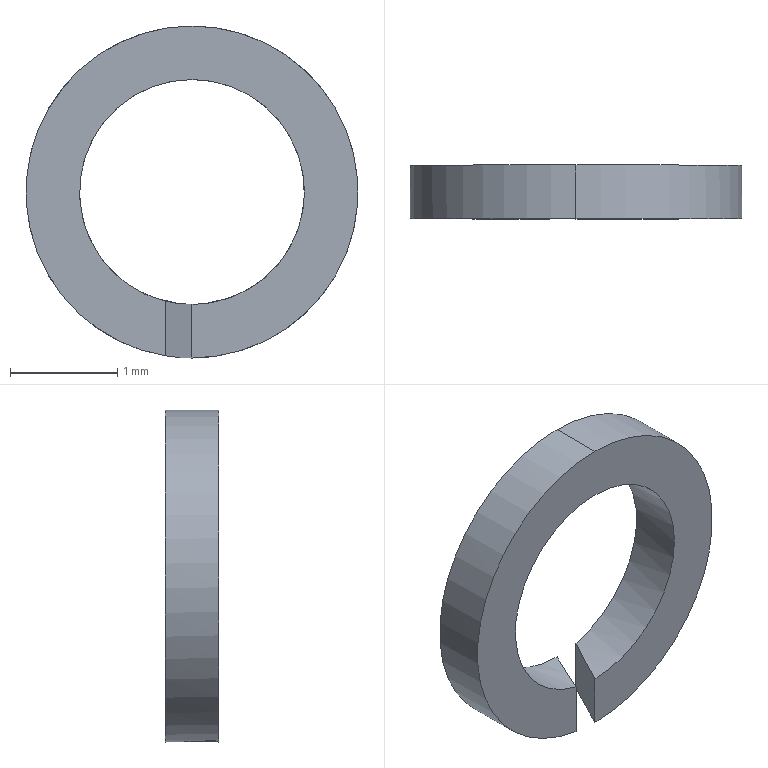Part | STEP file | _1-SO-80980001_1_1_1 | 1 solid | 8 faces | box 3.1 x 0.5 x 3.1 mm | volume 1.979 mm3 | cylinder 4 | plane 4 | commonest cylinder face diameters 2.1 x2 3.1 x2
STEP:
#1=CARTESIAN_POINT('',(0.,0.,0.));
#2=DIRECTION('',(0.,0.,1.));
#3=DIRECTION('',(1.,0.,0.));
#4=AXIS2_PLACEMENT_3D('',#1,#2,#3);
#5=CARTESIAN_POINT('',(-1.75,40.9,-83.78));
#6=VERTEX_POINT('',#5);
#7=CARTESIAN_POINT('',(-1.5,40.9,-80.7));
#8=VERTEX_POINT('',#7);
#9=CARTESIAN_POINT('',(-1.5,40.9,-82.25));
#10=DIRECTION('',(0.,1.,0.));
#11=DIRECTION('',(0.,0.,1.));
#12=AXIS2_PLACEMENT_3D('',#9,#10,#11);
#13=CIRCLE('',#12,1.55);
#14=CARTESIAN_POINT('',(-1.5,40.9,-82.25));
#15=DIRECTION('',(0.,1.,0.));
#16=DIRECTION('',(0.,0.,1.));
#17=AXIS2_PLACEMENT_3D('',#14,#15,#16);
#18=CYLINDRICAL_SURFACE('',#17,1.55);
#19=CARTESIAN_POINT('',(0.,0.));
#20=DIRECTION('',(1.,0.));
#21=VECTOR('',#20,1.);
#22=LINE('',#19,#21);
#23=(GEOMETRIC_REPRESENTATION_CONTEXT(2)PARAMETRIC_REPRESENTATION_CONTEXT()REPRESENTATION_CONTEXT('',''));
#24=DEFINITIONAL_REPRESENTATION('',(#22),#23);
#25=PCURVE('',#18,#24);
#26=CARTESIAN_POINT('',(-1.5,40.9,-82.25));
#27=DIRECTION('',(0.,1.,0.));
#28=DIRECTION('',(0.,0.,1.));
#29=AXIS2_PLACEMENT_3D('',#26,#27,#28);
#30=PLANE('',#29);
#31=CARTESIAN_POINT('',(0.,0.));
#32=DIRECTION('',(1.,0.));
#33=AXIS2_PLACEMENT_2D('',#31,#32);
#34=CIRCLE('',#33,1.55);
#35=(GEOMETRIC_REPRESENTATION_CONTEXT(2)PARAMETRIC_REPRESENTATION_CONTEXT()REPRESENTATION_CONTEXT('',''));
#36=DEFINITIONAL_REPRESENTATION('',(#34),#35);
#37=PCURVE('',#30,#36);
#38=SURFACE_CURVE('',#13,(#25,#37),.PCURVE_S1.);
#39=EDGE_CURVE('',#6,#8,#38,.T.);
#40=ORIENTED_EDGE('',*,*,#39,.T.);
#41=CARTESIAN_POINT('',(-1.5,41.4,-80.7));
#42=VERTEX_POINT('',#41);
#43=CARTESIAN_POINT('',(-1.5,40.9,-80.7));
#44=DIRECTION('',(0.,1.,0.));
#45=VECTOR('',#44,1.);
#46=LINE('',#43,#45);
#47=CARTESIAN_POINT('',(6.283,0.));
#48=DIRECTION('',(0.,1.));
#49=VECTOR('',#48,1.);
#50=LINE('',#47,#49);
#51=(GEOMETRIC_REPRESENTATION_CONTEXT(2)PARAMETRIC_REPRESENTATION_CONTEXT()REPRESENTATION_CONTEXT('',''));
#52=DEFINITIONAL_REPRESENTATION('',(#50),#51);
#53=PCURVE('',#18,#52);
#54=CARTESIAN_POINT('',(-1.5,40.9,-82.25));
#55=DIRECTION('',(0.,1.,0.));
#56=DIRECTION('',(0.,0.,1.));
#57=AXIS2_PLACEMENT_3D('',#54,#55,#56);
#58=CYLINDRICAL_SURFACE('',#57,1.55);
#59=CARTESIAN_POINT('',(0.,0.));
#60=DIRECTION('',(0.,1.));
#61=VECTOR('',#60,1.);
#62=LINE('',#59,#61);
#63=(GEOMETRIC_REPRESENTATION_CONTEXT(2)PARAMETRIC_REPRESENTATION_CONTEXT()REPRESENTATION_CONTEXT('',''));
#64=DEFINITIONAL_REPRESENTATION('',(#62),#63);
#65=PCURVE('',#58,#64);
#66=SURFACE_CURVE('',#46,(#53,#65),.PCURVE_S1.);
#67=EDGE_CURVE('',#8,#42,#66,.T.);
#68=ORIENTED_EDGE('',*,*,#67,.T.);
#69=CARTESIAN_POINT('',(-1.5,41.4,-83.8));
#70=VERTEX_POINT('',#69);
#71=CARTESIAN_POINT('',(-1.5,41.4,-82.25));
#72=DIRECTION('',(0.,1.,0.));
#73=DIRECTION('',(0.,0.,1.));
#74=AXIS2_PLACEMENT_3D('',#71,#72,#73);
#75=CIRCLE('',#74,1.55);
#76=CARTESIAN_POINT('',(0.,0.5));
#77=DIRECTION('',(1.,0.));
#78=VECTOR('',#77,1.);
#79=LINE('',#76,#78);
#80=(GEOMETRIC_REPRESENTATION_CONTEXT(2)PARAMETRIC_REPRESENTATION_CONTEXT()REPRESENTATION_CONTEXT('',''));
#81=DEFINITIONAL_REPRESENTATION('',(#79),#80);
#82=PCURVE('',#18,#81);
#83=CARTESIAN_POINT('',(-1.5,41.4,-82.25));
#84=DIRECTION('',(0.,1.,0.));
#85=DIRECTION('',(0.,0.,1.));
#86=AXIS2_PLACEMENT_3D('',#83,#84,#85);
#87=PLANE('',#86);
#88=CARTESIAN_POINT('',(0.,0.));
#89=DIRECTION('',(1.,0.));
#90=AXIS2_PLACEMENT_2D('',#88,#89);
#91=CIRCLE('',#90,1.55);
#92=(GEOMETRIC_REPRESENTATION_CONTEXT(2)PARAMETRIC_REPRESENTATION_CONTEXT()REPRESENTATION_CONTEXT('',''));
#93=DEFINITIONAL_REPRESENTATION('',(#91),#92);
#94=PCURVE('',#87,#93);
#95=SURFACE_CURVE('',#75,(#82,#94),.PCURVE_S1.);
#96=EDGE_CURVE('',#70,#42,#95,.T.);
#97=ORIENTED_EDGE('',*,*,#96,.F.);
#98=CARTESIAN_POINT('',(-1.5,41.4,-83.8));
#99=CARTESIAN_POINT('',(-1.584,41.232,-83.8));
#100=CARTESIAN_POINT('',(-1.667,41.065,-83.793));
#101=CARTESIAN_POINT('',(-1.75,40.9,-83.78));
#102=(BOUNDED_CURVE()B_SPLINE_CURVE(3,(#98,#99,#100,#101),.UNSPECIFIED.,.F.,.F.)B_SPLINE_CURVE_WITH_KNOTS((4,4),(1.571,1.733),.PIECEWISE_BEZIER_KNOTS.)CURVE()GEOMETRIC_REPRESENTATION_ITEM()RATIONAL_B_SPLINE_CURVE((1.,0.9978,0.9978,1.))REPRESENTATION_ITEM(''));
#103=CARTESIAN_POINT('',(3.142,0.5));
#104=CARTESIAN_POINT('',(3.144,0.4924));
#105=CARTESIAN_POINT('',(3.149,0.4772));
#106=CARTESIAN_POINT('',(3.156,0.4544));
#107=CARTESIAN_POINT('',(3.164,0.4316));
#108=CARTESIAN_POINT('',(3.171,0.4088));
#109=CARTESIAN_POINT('',(3.178,0.3859));
#110=CARTESIAN_POINT('',(3.186,0.3631));
#111=CARTESIAN_POINT('',(3.193,0.3403));
#112=CARTESIAN_POINT('',(3.2,0.3175));
#113=CARTESIAN_POINT('',(3.208,0.2947));
#114=CARTESIAN_POINT('',(3.215,0.2719));
#115=CARTESIAN_POINT('',(3.223,0.2492));
#116=CARTESIAN_POINT('',(3.23,0.2264));
#117=CARTESIAN_POINT('',(3.237,0.2037));
#118=CARTESIAN_POINT('',(3.245,0.181));
#119=CARTESIAN_POINT('',(3.252,0.1582));
#120=CARTESIAN_POINT('',(3.259,0.1356));
#121=CARTESIAN_POINT('',(3.267,0.1129));
#122=CARTESIAN_POINT('',(3.274,0.09026));
#123=CARTESIAN_POINT('',(3.282,0.06765));
#124=CARTESIAN_POINT('',(3.289,0.04507));
#125=CARTESIAN_POINT('',(3.296,0.02251));
#126=CARTESIAN_POINT('',(3.301,0.007501));
#127=CARTESIAN_POINT('',(3.304,0.));
#128=B_SPLINE_CURVE_WITH_KNOTS('',3,(#103,#104,#105,#106,#107,#108,#109,#110,#111,#112,#113,#114,#115,#116,#117,#118,#119,#120,#121,#122,#123,#124,#125,#126,#127),.UNSPECIFIED.,.F.,.F.,(4,1,1,1,1,1,1,1,1,1,1,1,1,1,1,1,1,1,1,1,1,1,4),(1.571,1.578,1.586,1.593,1.6,1.608,1.615,1.622,1.63,1.637,1.644,1.652,1.659,1.667,1.674,1.681,1.689,1.696,1.703,1.711,1.718,1.725,1.733),.QUASI_UNIFORM_KNOTS.);
#129=(GEOMETRIC_REPRESENTATION_CONTEXT(2)PARAMETRIC_REPRESENTATION_CONTEXT()REPRESENTATION_CONTEXT('',''));
#130=DEFINITIONAL_REPRESENTATION('',(#128),#129);
#131=PCURVE('',#18,#130);
#132=CARTESIAN_POINT('',(-1.75,40.9,-82.25));
#133=DIRECTION('',(-0.8944,0.4472,0.));
#134=DIRECTION('',(-0.4472,-0.8944,0.));
#135=AXIS2_PLACEMENT_3D('',#132,#133,#134);
#136=PLANE('',#135);
#137=CARTESIAN_POINT('',(-0.559,-1.55));
#138=CARTESIAN_POINT('',(-0.3717,-1.55));
#139=CARTESIAN_POINT('',(-0.1849,-1.543));
#140=CARTESIAN_POINT('',(0.,-1.53));
#141=(BOUNDED_CURVE()B_SPLINE_CURVE(3,(#137,#138,#139,#140),.UNSPECIFIED.,.F.,.F.)B_SPLINE_CURVE_WITH_KNOTS((4,4),(1.571,1.733),.PIECEWISE_BEZIER_KNOTS.)CURVE()GEOMETRIC_REPRESENTATION_ITEM()RATIONAL_B_SPLINE_CURVE((1.,0.9978,0.9978,1.))REPRESENTATION_ITEM(''));
#142=(GEOMETRIC_REPRESENTATION_CONTEXT(2)PARAMETRIC_REPRESENTATION_CONTEXT()REPRESENTATION_CONTEXT('',''));
#143=DEFINITIONAL_REPRESENTATION('',(#141),#142);
#144=PCURVE('',#136,#143);
#145=SURFACE_CURVE('',#102,(#131,#144),.PCURVE_S1.);
#146=EDGE_CURVE('',#70,#6,#145,.T.);
#147=ORIENTED_EDGE('',*,*,#146,.T.);
#148=EDGE_LOOP('',(#40,#68,#97,#147));
#149=FACE_BOUND('',#148,.T.);
#150=ADVANCED_FACE('',(#149),#18,.T.);
#151=CARTESIAN_POINT('',(-1.5,40.9,-83.3));
#152=VERTEX_POINT('',#151);
#153=CARTESIAN_POINT('',(-1.25,41.4,-83.27));
#154=VERTEX_POINT('',#153);
#155=CARTESIAN_POINT('',(-1.5,40.9,-83.3));
#156=CARTESIAN_POINT('',(-1.416,41.069,-83.3));
#157=CARTESIAN_POINT('',(-1.332,41.236,-83.29));
#158=CARTESIAN_POINT('',(-1.25,41.4,-83.27));
#159=(BOUNDED_CURVE()B_SPLINE_CURVE(3,(#155,#156,#157,#158),.UNSPECIFIED.,.F.,.F.)B_SPLINE_CURVE_WITH_KNOTS((4,4),(4.712,4.953),.PIECEWISE_BEZIER_KNOTS.)CURVE()GEOMETRIC_REPRESENTATION_ITEM()RATIONAL_B_SPLINE_CURVE((1.,0.9952,0.9952,1.))REPRESENTATION_ITEM(''));
#160=CARTESIAN_POINT('',(-1.5,40.9,-82.25));
#161=DIRECTION('',(0.,1.,0.));
#162=DIRECTION('',(0.,0.,1.));
#163=AXIS2_PLACEMENT_3D('',#160,#161,#162);
#164=CYLINDRICAL_SURFACE('',#163,1.05);
#165=CARTESIAN_POINT('',(3.142,0.));
#166=CARTESIAN_POINT('',(3.138,0.007631));
#167=CARTESIAN_POINT('',(3.131,0.0229));
#168=CARTESIAN_POINT('',(3.12,0.04581));
#169=CARTESIAN_POINT('',(3.109,0.06873));
#170=CARTESIAN_POINT('',(3.098,0.09165));
#171=CARTESIAN_POINT('',(3.087,0.1146));
#172=CARTESIAN_POINT('',(3.076,0.1375));
#173=CARTESIAN_POINT('',(3.065,0.1604));
#174=CARTESIAN_POINT('',(3.054,0.1833));
#175=CARTESIAN_POINT('',(3.043,0.2061));
#176=CARTESIAN_POINT('',(3.032,0.229));
#177=CARTESIAN_POINT('',(3.021,0.2518));
#178=CARTESIAN_POINT('',(3.01,0.2746));
#179=CARTESIAN_POINT('',(3.,0.2974));
#180=CARTESIAN_POINT('',(2.989,0.3201));
#181=CARTESIAN_POINT('',(2.978,0.3428));
#182=CARTESIAN_POINT('',(2.967,0.3654));
#183=CARTESIAN_POINT('',(2.956,0.388));
#184=CARTESIAN_POINT('',(2.945,0.4105));
#185=CARTESIAN_POINT('',(2.934,0.433));
#186=CARTESIAN_POINT('',(2.923,0.4554));
#187=CARTESIAN_POINT('',(2.912,0.4777));
#188=CARTESIAN_POINT('',(2.905,0.4926));
#189=CARTESIAN_POINT('',(2.901,0.5));
#190=B_SPLINE_CURVE_WITH_KNOTS('',3,(#165,#166,#167,#168,#169,#170,#171,#172,#173,#174,#175,#176,#177,#178,#179,#180,#181,#182,#183,#184,#185,#186,#187,#188,#189),.UNSPECIFIED.,.F.,.F.,(4,1,1,1,1,1,1,1,1,1,1,1,1,1,1,1,1,1,1,1,1,1,4),(4.712,4.723,4.734,4.745,4.756,4.767,4.778,4.789,4.8,4.811,4.822,4.833,4.844,4.854,4.865,4.876,4.887,4.898,4.909,4.92,4.931,4.942,4.953),.QUASI_UNIFORM_KNOTS.);
#191=(GEOMETRIC_REPRESENTATION_CONTEXT(2)PARAMETRIC_REPRESENTATION_CONTEXT()REPRESENTATION_CONTEXT('',''));
#192=DEFINITIONAL_REPRESENTATION('',(#190),#191);
#193=PCURVE('',#164,#192);
#194=CARTESIAN_POINT('',(-1.25,41.4,-82.25));
#195=DIRECTION('',(0.8944,-0.4472,0.));
#196=DIRECTION('',(0.4472,0.8944,0.));
#197=AXIS2_PLACEMENT_3D('',#194,#195,#196);
#198=PLANE('',#197);
#199=CARTESIAN_POINT('',(-0.559,-1.05));
#200=CARTESIAN_POINT('',(-0.3704,-1.05));
#201=CARTESIAN_POINT('',(-0.1832,-1.04));
#202=CARTESIAN_POINT('',(0.,-1.02));
#203=(BOUNDED_CURVE()B_SPLINE_CURVE(3,(#199,#200,#201,#202),.UNSPECIFIED.,.F.,.F.)B_SPLINE_CURVE_WITH_KNOTS((4,4),(4.712,4.953),.PIECEWISE_BEZIER_KNOTS.)CURVE()GEOMETRIC_REPRESENTATION_ITEM()RATIONAL_B_SPLINE_CURVE((1.,0.9952,0.9952,1.))REPRESENTATION_ITEM(''));
#204=(GEOMETRIC_REPRESENTATION_CONTEXT(2)PARAMETRIC_REPRESENTATION_CONTEXT()REPRESENTATION_CONTEXT('',''));
#205=DEFINITIONAL_REPRESENTATION('',(#203),#204);
#206=PCURVE('',#198,#205);
#207=SURFACE_CURVE('',#159,(#193,#206),.PCURVE_S1.);
#208=EDGE_CURVE('',#152,#154,#207,.T.);
#209=ORIENTED_EDGE('',*,*,#208,.T.);
#210=CARTESIAN_POINT('',(-1.5,41.4,-81.2));
#211=VERTEX_POINT('',#210);
#212=CARTESIAN_POINT('',(-1.5,41.4,-82.25));
#213=DIRECTION('',(0.,-1.,0.));
#214=DIRECTION('',(0.,0.,1.));
#215=AXIS2_PLACEMENT_3D('',#212,#213,#214);
#216=CIRCLE('',#215,1.05);
#217=CARTESIAN_POINT('',(6.283,0.5));
#218=DIRECTION('',(-1.,0.));
#219=VECTOR('',#218,1.);
#220=LINE('',#217,#219);
#221=(GEOMETRIC_REPRESENTATION_CONTEXT(2)PARAMETRIC_REPRESENTATION_CONTEXT()REPRESENTATION_CONTEXT('',''));
#222=DEFINITIONAL_REPRESENTATION('',(#220),#221);
#223=PCURVE('',#164,#222);
#224=CARTESIAN_POINT('',(1.05,0.));
#225=CARTESIAN_POINT('',(1.05,-1.819));
#226=CARTESIAN_POINT('',(-0.525,-0.9093));
#227=CARTESIAN_POINT('',(-2.1,0.));
#228=CARTESIAN_POINT('',(-0.525,0.9093));
#229=CARTESIAN_POINT('',(1.05,1.819));
#230=CARTESIAN_POINT('',(1.05,0.));
#231=(BOUNDED_CURVE()B_SPLINE_CURVE(2,(#224,#225,#226,#227,#228,#229,#230),.UNSPECIFIED.,.T.,.F.)B_SPLINE_CURVE_WITH_KNOTS((1,2,2,2,2,1),(-2.094,0.,2.094,4.189,6.283,8.378),.UNSPECIFIED.)CURVE()GEOMETRIC_REPRESENTATION_ITEM()RATIONAL_B_SPLINE_CURVE((1.,0.5,1.,0.5,1.,0.5,1.))REPRESENTATION_ITEM(''));
#232=(GEOMETRIC_REPRESENTATION_CONTEXT(2)PARAMETRIC_REPRESENTATION_CONTEXT()REPRESENTATION_CONTEXT('',''));
#233=DEFINITIONAL_REPRESENTATION('',(#231),#232);
#234=PCURVE('',#87,#233);
#235=SURFACE_CURVE('',#216,(#223,#234),.PCURVE_S1.);
#236=EDGE_CURVE('',#154,#211,#235,.T.);
#237=ORIENTED_EDGE('',*,*,#236,.T.);
#238=CARTESIAN_POINT('',(-1.5,40.9,-81.2));
#239=VERTEX_POINT('',#238);
#240=CARTESIAN_POINT('',(-1.5,40.9,-81.2));
#241=DIRECTION('',(0.,1.,0.));
#242=VECTOR('',#241,1.);
#243=LINE('',#240,#242);
#244=CARTESIAN_POINT('',(0.,0.));
#245=DIRECTION('',(0.,1.));
#246=VECTOR('',#245,1.);
#247=LINE('',#244,#246);
#248=(GEOMETRIC_REPRESENTATION_CONTEXT(2)PARAMETRIC_REPRESENTATION_CONTEXT()REPRESENTATION_CONTEXT('',''));
#249=DEFINITIONAL_REPRESENTATION('',(#247),#248);
#250=PCURVE('',#164,#249);
#251=CARTESIAN_POINT('',(-1.5,40.9,-82.25));
#252=DIRECTION('',(0.,1.,0.));
#253=DIRECTION('',(0.,0.,1.));
#254=AXIS2_PLACEMENT_3D('',#251,#252,#253);
#255=CYLINDRICAL_SURFACE('',#254,1.05);
#256=CARTESIAN_POINT('',(6.283,0.));
#257=DIRECTION('',(0.,1.));
#258=VECTOR('',#257,1.);
#259=LINE('',#256,#258);
#260=(GEOMETRIC_REPRESENTATION_CONTEXT(2)PARAMETRIC_REPRESENTATION_CONTEXT()REPRESENTATION_CONTEXT('',''));
#261=DEFINITIONAL_REPRESENTATION('',(#259),#260);
#262=PCURVE('',#255,#261);
#263=SURFACE_CURVE('',#243,(#250,#262),.PCURVE_S1.);
#264=EDGE_CURVE('',#239,#211,#263,.T.);
#265=ORIENTED_EDGE('',*,*,#264,.F.);
#266=CARTESIAN_POINT('',(-1.5,40.9,-82.25));
#267=DIRECTION('',(0.,1.,0.));
#268=DIRECTION('',(0.,0.,1.));
#269=AXIS2_PLACEMENT_3D('',#266,#267,#268);
#270=CIRCLE('',#269,1.05);
#271=CARTESIAN_POINT('',(0.,0.));
#272=DIRECTION('',(1.,0.));
#273=VECTOR('',#272,1.);
#274=LINE('',#271,#273);
#275=(GEOMETRIC_REPRESENTATION_CONTEXT(2)PARAMETRIC_REPRESENTATION_CONTEXT()REPRESENTATION_CONTEXT('',''));
#276=DEFINITIONAL_REPRESENTATION('',(#274),#275);
#277=PCURVE('',#164,#276);
#278=CARTESIAN_POINT('',(0.,0.));
#279=DIRECTION('',(1.,0.));
#280=AXIS2_PLACEMENT_2D('',#278,#279);
#281=CIRCLE('',#280,1.05);
#282=(GEOMETRIC_REPRESENTATION_CONTEXT(2)PARAMETRIC_REPRESENTATION_CONTEXT()REPRESENTATION_CONTEXT('',''));
#283=DEFINITIONAL_REPRESENTATION('',(#281),#282);
#284=PCURVE('',#30,#283);
#285=SURFACE_CURVE('',#270,(#277,#284),.PCURVE_S1.);
#286=EDGE_CURVE('',#239,#152,#285,.T.);
#287=ORIENTED_EDGE('',*,*,#286,.T.);
#288=EDGE_LOOP('',(#209,#237,#265,#287));
#289=FACE_BOUND('',#288,.F.);
#290=ADVANCED_FACE('',(#289),#164,.F.);
#291=ORIENTED_EDGE('',*,*,#96,.T.);
#292=CARTESIAN_POINT('',(-1.25,41.4,-83.78));
#293=VERTEX_POINT('',#292);
#294=CARTESIAN_POINT('',(-1.5,41.4,-82.25));
#295=DIRECTION('',(0.,1.,0.));
#296=DIRECTION('',(0.,0.,1.));
#297=AXIS2_PLACEMENT_3D('',#294,#295,#296);
#298=CIRCLE('',#297,1.55);
#299=CARTESIAN_POINT('',(0.,0.));
#300=DIRECTION('',(1.,0.));
#301=AXIS2_PLACEMENT_2D('',#299,#300);
#302=CIRCLE('',#301,1.55);
#303=(GEOMETRIC_REPRESENTATION_CONTEXT(2)PARAMETRIC_REPRESENTATION_CONTEXT()REPRESENTATION_CONTEXT('',''));
#304=DEFINITIONAL_REPRESENTATION('',(#302),#303);
#305=PCURVE('',#87,#304);
#306=CARTESIAN_POINT('',(0.,0.5));
#307=DIRECTION('',(1.,0.));
#308=VECTOR('',#307,1.);
#309=LINE('',#306,#308);
#310=(GEOMETRIC_REPRESENTATION_CONTEXT(2)PARAMETRIC_REPRESENTATION_CONTEXT()REPRESENTATION_CONTEXT('',''));
#311=DEFINITIONAL_REPRESENTATION('',(#309),#310);
#312=PCURVE('',#58,#311);
#313=SURFACE_CURVE('',#298,(#305,#312),.PCURVE_S1.);
#314=EDGE_CURVE('',#42,#293,#313,.T.);
#315=ORIENTED_EDGE('',*,*,#314,.T.);
#316=CARTESIAN_POINT('',(-1.25,41.4,-82.25));
#317=DIRECTION('',(0.,0.,1.));
#318=VECTOR('',#317,1.);
#319=LINE('',#316,#318);
#320=CARTESIAN_POINT('',(0.,0.25));
#321=DIRECTION('',(1.,0.));
#322=VECTOR('',#321,1.);
#323=LINE('',#320,#322);
#324=(GEOMETRIC_REPRESENTATION_CONTEXT(2)PARAMETRIC_REPRESENTATION_CONTEXT()REPRESENTATION_CONTEXT('',''));
#325=DEFINITIONAL_REPRESENTATION('',(#323),#324);
#326=PCURVE('',#87,#325);
#327=CARTESIAN_POINT('',(0.,0.));
#328=DIRECTION('',(0.,1.));
#329=VECTOR('',#328,1.);
#330=LINE('',#327,#329);
#331=(GEOMETRIC_REPRESENTATION_CONTEXT(2)PARAMETRIC_REPRESENTATION_CONTEXT()REPRESENTATION_CONTEXT('',''));
#332=DEFINITIONAL_REPRESENTATION('',(#330),#331);
#333=PCURVE('',#198,#332);
#334=SURFACE_CURVE('',#319,(#326,#333),.PCURVE_S1.);
#335=EDGE_CURVE('',#293,#154,#334,.T.);
#336=ORIENTED_EDGE('',*,*,#335,.T.);
#337=ORIENTED_EDGE('',*,*,#236,.T.);
#338=CARTESIAN_POINT('',(-1.5,41.4,-83.3));
#339=VERTEX_POINT('',#338);
#340=CARTESIAN_POINT('',(-1.5,41.4,-82.25));
#341=DIRECTION('',(0.,-1.,0.));
#342=DIRECTION('',(0.,0.,1.));
#343=AXIS2_PLACEMENT_3D('',#340,#341,#342);
#344=CIRCLE('',#343,1.05);
#345=CARTESIAN_POINT('',(1.05,0.));
#346=CARTESIAN_POINT('',(1.05,-1.819));
#347=CARTESIAN_POINT('',(-0.525,-0.9093));
#348=CARTESIAN_POINT('',(-2.1,0.));
#349=CARTESIAN_POINT('',(-0.525,0.9093));
#350=CARTESIAN_POINT('',(1.05,1.819));
#351=CARTESIAN_POINT('',(1.05,0.));
#352=(BOUNDED_CURVE()B_SPLINE_CURVE(2,(#345,#346,#347,#348,#349,#350,#351),.UNSPECIFIED.,.T.,.F.)B_SPLINE_CURVE_WITH_KNOTS((1,2,2,2,2,1),(-2.094,0.,2.094,4.189,6.283,8.378),.UNSPECIFIED.)CURVE()GEOMETRIC_REPRESENTATION_ITEM()RATIONAL_B_SPLINE_CURVE((1.,0.5,1.,0.5,1.,0.5,1.))REPRESENTATION_ITEM(''));
#353=(GEOMETRIC_REPRESENTATION_CONTEXT(2)PARAMETRIC_REPRESENTATION_CONTEXT()REPRESENTATION_CONTEXT('',''));
#354=DEFINITIONAL_REPRESENTATION('',(#352),#353);
#355=PCURVE('',#87,#354);
#356=CARTESIAN_POINT('',(6.283,0.5));
#357=DIRECTION('',(-1.,0.));
#358=VECTOR('',#357,1.);
#359=LINE('',#356,#358);
#360=(GEOMETRIC_REPRESENTATION_CONTEXT(2)PARAMETRIC_REPRESENTATION_CONTEXT()REPRESENTATION_CONTEXT('',''));
#361=DEFINITIONAL_REPRESENTATION('',(#359),#360);
#362=PCURVE('',#255,#361);
#363=SURFACE_CURVE('',#344,(#355,#362),.PCURVE_S1.);
#364=EDGE_CURVE('',#211,#339,#363,.T.);
#365=ORIENTED_EDGE('',*,*,#364,.T.);
#366=CARTESIAN_POINT('',(-1.5,41.4,-82.25));
#367=DIRECTION('',(0.,0.,-1.));
#368=VECTOR('',#367,1.);
#369=LINE('',#366,#368);
#370=CARTESIAN_POINT('',(0.,0.));
#371=DIRECTION('',(-1.,0.));
#372=VECTOR('',#371,1.);
#373=LINE('',#370,#372);
#374=(GEOMETRIC_REPRESENTATION_CONTEXT(2)PARAMETRIC_REPRESENTATION_CONTEXT()REPRESENTATION_CONTEXT('',''));
#375=DEFINITIONAL_REPRESENTATION('',(#373),#374);
#376=PCURVE('',#87,#375);
#377=CARTESIAN_POINT('',(-0.559,0.));
#378=DIRECTION('',(0.,-1.));
#379=VECTOR('',#378,1.);
#380=LINE('',#377,#379);
#381=(GEOMETRIC_REPRESENTATION_CONTEXT(2)PARAMETRIC_REPRESENTATION_CONTEXT()REPRESENTATION_CONTEXT('',''));
#382=DEFINITIONAL_REPRESENTATION('',(#380),#381);
#383=PCURVE('',#136,#382);
#384=SURFACE_CURVE('',#369,(#376,#383),.PCURVE_S1.);
#385=EDGE_CURVE('',#339,#70,#384,.T.);
#386=ORIENTED_EDGE('',*,*,#385,.T.);
#387=EDGE_LOOP('',(#291,#315,#336,#337,#365,#386));
#388=FACE_BOUND('',#387,.T.);
#389=ADVANCED_FACE('',(#388),#87,.T.);
#390=ORIENTED_EDGE('',*,*,#67,.F.);
#391=CARTESIAN_POINT('',(-1.5,40.9,-83.8));
#392=VERTEX_POINT('',#391);
#393=CARTESIAN_POINT('',(-1.5,40.9,-82.25));
#394=DIRECTION('',(0.,1.,0.));
#395=DIRECTION('',(0.,0.,1.));
#396=AXIS2_PLACEMENT_3D('',#393,#394,#395);
#397=CIRCLE('',#396,1.55);
#398=CARTESIAN_POINT('',(0.,0.));
#399=DIRECTION('',(1.,0.));
#400=VECTOR('',#399,1.);
#401=LINE('',#398,#400);
#402=(GEOMETRIC_REPRESENTATION_CONTEXT(2)PARAMETRIC_REPRESENTATION_CONTEXT()REPRESENTATION_CONTEXT('',''));
#403=DEFINITIONAL_REPRESENTATION('',(#401),#402);
#404=PCURVE('',#58,#403);
#405=CARTESIAN_POINT('',(0.,0.));
#406=DIRECTION('',(1.,0.));
#407=AXIS2_PLACEMENT_2D('',#405,#406);
#408=CIRCLE('',#407,1.55);
#409=(GEOMETRIC_REPRESENTATION_CONTEXT(2)PARAMETRIC_REPRESENTATION_CONTEXT()REPRESENTATION_CONTEXT('',''));
#410=DEFINITIONAL_REPRESENTATION('',(#408),#409);
#411=PCURVE('',#30,#410);
#412=SURFACE_CURVE('',#397,(#404,#411),.PCURVE_S1.);
#413=EDGE_CURVE('',#8,#392,#412,.T.);
#414=ORIENTED_EDGE('',*,*,#413,.T.);
#415=CARTESIAN_POINT('',(-1.5,40.9,-83.8));
#416=CARTESIAN_POINT('',(-1.416,41.068,-83.8));
#417=CARTESIAN_POINT('',(-1.333,41.235,-83.793));
#418=CARTESIAN_POINT('',(-1.25,41.4,-83.78));
#419=(BOUNDED_CURVE()B_SPLINE_CURVE(3,(#415,#416,#417,#418),.UNSPECIFIED.,.F.,.F.)B_SPLINE_CURVE_WITH_KNOTS((4,4),(4.712,4.874),.PIECEWISE_BEZIER_KNOTS.)CURVE()GEOMETRIC_REPRESENTATION_ITEM()RATIONAL_B_SPLINE_CURVE((1.,0.9978,0.9978,1.))REPRESENTATION_ITEM(''));
#420=CARTESIAN_POINT('',(3.142,0.));
#421=CARTESIAN_POINT('',(3.139,0.007601));
#422=CARTESIAN_POINT('',(3.134,0.0228));
#423=CARTESIAN_POINT('',(3.127,0.04561));
#424=CARTESIAN_POINT('',(3.12,0.06843));
#425=CARTESIAN_POINT('',(3.112,0.09124));
#426=CARTESIAN_POINT('',(3.105,0.1141));
#427=CARTESIAN_POINT('',(3.097,0.1369));
#428=CARTESIAN_POINT('',(3.09,0.1597));
#429=CARTESIAN_POINT('',(3.083,0.1825));
#430=CARTESIAN_POINT('',(3.075,0.2053));
#431=CARTESIAN_POINT('',(3.068,0.2281));
#432=CARTESIAN_POINT('',(3.061,0.2508));
#433=CARTESIAN_POINT('',(3.053,0.2736));
#434=CARTESIAN_POINT('',(3.046,0.2963));
#435=CARTESIAN_POINT('',(3.038,0.319));
#436=CARTESIAN_POINT('',(3.031,0.3418));
#437=CARTESIAN_POINT('',(3.024,0.3644));
#438=CARTESIAN_POINT('',(3.016,0.3871));
#439=CARTESIAN_POINT('',(3.009,0.4097));
#440=CARTESIAN_POINT('',(3.002,0.4324));
#441=CARTESIAN_POINT('',(2.994,0.4549));
#442=CARTESIAN_POINT('',(2.987,0.4775));
#443=CARTESIAN_POINT('',(2.982,0.4925));
#444=CARTESIAN_POINT('',(2.98,0.5));
#445=B_SPLINE_CURVE_WITH_KNOTS('',3,(#420,#421,#422,#423,#424,#425,#426,#427,#428,#429,#430,#431,#432,#433,#434,#435,#436,#437,#438,#439,#440,#441,#442,#443,#444),.UNSPECIFIED.,.F.,.F.,(4,1,1,1,1,1,1,1,1,1,1,1,1,1,1,1,1,1,1,1,1,1,4),(4.712,4.72,4.727,4.734,4.742,4.749,4.757,4.764,4.771,4.779,4.786,4.793,4.801,4.808,4.815,4.823,4.83,4.838,4.845,4.852,4.86,4.867,4.874),.QUASI_UNIFORM_KNOTS.);
#446=(GEOMETRIC_REPRESENTATION_CONTEXT(2)PARAMETRIC_REPRESENTATION_CONTEXT()REPRESENTATION_CONTEXT('',''));
#447=DEFINITIONAL_REPRESENTATION('',(#445),#446);
#448=PCURVE('',#58,#447);
#449=CARTESIAN_POINT('',(-0.559,-1.55));
#450=CARTESIAN_POINT('',(-0.3717,-1.55));
#451=CARTESIAN_POINT('',(-0.1849,-1.543));
#452=CARTESIAN_POINT('',(0.,-1.53));
#453=(BOUNDED_CURVE()B_SPLINE_CURVE(3,(#449,#450,#451,#452),.UNSPECIFIED.,.F.,.F.)B_SPLINE_CURVE_WITH_KNOTS((4,4),(4.712,4.874),.PIECEWISE_BEZIER_KNOTS.)CURVE()GEOMETRIC_REPRESENTATION_ITEM()RATIONAL_B_SPLINE_CURVE((1.,0.9978,0.9978,1.))REPRESENTATION_ITEM(''));
#454=(GEOMETRIC_REPRESENTATION_CONTEXT(2)PARAMETRIC_REPRESENTATION_CONTEXT()REPRESENTATION_CONTEXT('',''));
#455=DEFINITIONAL_REPRESENTATION('',(#453),#454);
#456=PCURVE('',#198,#455);
#457=SURFACE_CURVE('',#419,(#448,#456),.PCURVE_S1.);
#458=EDGE_CURVE('',#392,#293,#457,.T.);
#459=ORIENTED_EDGE('',*,*,#458,.T.);
#460=ORIENTED_EDGE('',*,*,#314,.F.);
#461=EDGE_LOOP('',(#390,#414,#459,#460));
#462=FACE_BOUND('',#461,.T.);
#463=ADVANCED_FACE('',(#462),#58,.T.);
#464=CARTESIAN_POINT('',(-1.75,40.9,-83.27));
#465=VERTEX_POINT('',#464);
#466=CARTESIAN_POINT('',(-1.75,40.9,-83.27));
#467=CARTESIAN_POINT('',(-1.668,41.064,-83.29));
#468=CARTESIAN_POINT('',(-1.584,41.231,-83.3));
#469=CARTESIAN_POINT('',(-1.5,41.4,-83.3));
#470=(BOUNDED_CURVE()B_SPLINE_CURVE(3,(#466,#467,#468,#469),.UNSPECIFIED.,.F.,.F.)B_SPLINE_CURVE_WITH_KNOTS((4,4),(4.472,4.712),.PIECEWISE_BEZIER_KNOTS.)CURVE()GEOMETRIC_REPRESENTATION_ITEM()RATIONAL_B_SPLINE_CURVE((1.,0.9952,0.9952,1.))REPRESENTATION_ITEM(''));
#471=CARTESIAN_POINT('',(0.,-1.02));
#472=CARTESIAN_POINT('',(-0.1832,-1.04));
#473=CARTESIAN_POINT('',(-0.3704,-1.05));
#474=CARTESIAN_POINT('',(-0.559,-1.05));
#475=(BOUNDED_CURVE()B_SPLINE_CURVE(3,(#471,#472,#473,#474),.UNSPECIFIED.,.F.,.F.)B_SPLINE_CURVE_WITH_KNOTS((4,4),(4.472,4.712),.PIECEWISE_BEZIER_KNOTS.)CURVE()GEOMETRIC_REPRESENTATION_ITEM()RATIONAL_B_SPLINE_CURVE((1.,0.9952,0.9952,1.))REPRESENTATION_ITEM(''));
#476=(GEOMETRIC_REPRESENTATION_CONTEXT(2)PARAMETRIC_REPRESENTATION_CONTEXT()REPRESENTATION_CONTEXT('',''));
#477=DEFINITIONAL_REPRESENTATION('',(#475),#476);
#478=PCURVE('',#136,#477);
#479=CARTESIAN_POINT('',(3.382,0.));
#480=CARTESIAN_POINT('',(3.378,0.007411));
#481=CARTESIAN_POINT('',(3.371,0.02226));
#482=CARTESIAN_POINT('',(3.36,0.0446));
#483=CARTESIAN_POINT('',(3.349,0.06701));
#484=CARTESIAN_POINT('',(3.338,0.08948));
#485=CARTESIAN_POINT('',(3.327,0.112));
#486=CARTESIAN_POINT('',(3.316,0.1346));
#487=CARTESIAN_POINT('',(3.306,0.1572));
#488=CARTESIAN_POINT('',(3.295,0.1799));
#489=CARTESIAN_POINT('',(3.284,0.2026));
#490=CARTESIAN_POINT('',(3.273,0.2254));
#491=CARTESIAN_POINT('',(3.262,0.2482));
#492=CARTESIAN_POINT('',(3.251,0.271));
#493=CARTESIAN_POINT('',(3.24,0.2939));
#494=CARTESIAN_POINT('',(3.229,0.3167));
#495=CARTESIAN_POINT('',(3.218,0.3396));
#496=CARTESIAN_POINT('',(3.207,0.3625));
#497=CARTESIAN_POINT('',(3.196,0.3854));
#498=CARTESIAN_POINT('',(3.185,0.4084));
#499=CARTESIAN_POINT('',(3.174,0.4313));
#500=CARTESIAN_POINT('',(3.163,0.4542));
#501=CARTESIAN_POINT('',(3.152,0.4771));
#502=CARTESIAN_POINT('',(3.145,0.4924));
#503=CARTESIAN_POINT('',(3.142,0.5));
#504=B_SPLINE_CURVE_WITH_KNOTS('',3,(#479,#480,#481,#482,#483,#484,#485,#486,#487,#488,#489,#490,#491,#492,#493,#494,#495,#496,#497,#498,#499,#500,#501,#502,#503),.UNSPECIFIED.,.F.,.F.,(4,1,1,1,1,1,1,1,1,1,1,1,1,1,1,1,1,1,1,1,1,1,4),(4.472,4.483,4.494,4.505,4.516,4.527,4.538,4.548,4.559,4.57,4.581,4.592,4.603,4.614,4.625,4.636,4.647,4.658,4.669,4.68,4.691,4.701,4.712),.QUASI_UNIFORM_KNOTS.);
#505=(GEOMETRIC_REPRESENTATION_CONTEXT(2)PARAMETRIC_REPRESENTATION_CONTEXT()REPRESENTATION_CONTEXT('',''));
#506=DEFINITIONAL_REPRESENTATION('',(#504),#505);
#507=PCURVE('',#255,#506);
#508=SURFACE_CURVE('',#470,(#478,#507),.PCURVE_S1.);
#509=EDGE_CURVE('',#465,#339,#508,.T.);
#510=ORIENTED_EDGE('',*,*,#509,.F.);
#511=CARTESIAN_POINT('',(-1.75,40.9,-82.25));
#512=DIRECTION('',(0.,0.,1.));
#513=VECTOR('',#512,1.);
#514=LINE('',#511,#513);
#515=CARTESIAN_POINT('',(0.,0.));
#516=DIRECTION('',(0.,1.));
#517=VECTOR('',#516,1.);
#518=LINE('',#515,#517);
#519=(GEOMETRIC_REPRESENTATION_CONTEXT(2)PARAMETRIC_REPRESENTATION_CONTEXT()REPRESENTATION_CONTEXT('',''));
#520=DEFINITIONAL_REPRESENTATION('',(#518),#519);
#521=PCURVE('',#136,#520);
#522=CARTESIAN_POINT('',(0.,-0.25));
#523=DIRECTION('',(1.,0.));
#524=VECTOR('',#523,1.);
#525=LINE('',#522,#524);
#526=(GEOMETRIC_REPRESENTATION_CONTEXT(2)PARAMETRIC_REPRESENTATION_CONTEXT()REPRESENTATION_CONTEXT('',''));
#527=DEFINITIONAL_REPRESENTATION('',(#525),#526);
#528=PCURVE('',#30,#527);
#529=SURFACE_CURVE('',#514,(#521,#528),.PCURVE_S1.);
#530=EDGE_CURVE('',#6,#465,#529,.T.);
#531=ORIENTED_EDGE('',*,*,#530,.F.);
#532=ORIENTED_EDGE('',*,*,#146,.F.);
#533=ORIENTED_EDGE('',*,*,#385,.F.);
#534=EDGE_LOOP('',(#510,#531,#532,#533));
#535=FACE_BOUND('',#534,.T.);
#536=ADVANCED_FACE('',(#535),#136,.F.);
#537=ORIENTED_EDGE('',*,*,#364,.T.);
#538=ORIENTED_EDGE('',*,*,#509,.F.);
#539=CARTESIAN_POINT('',(-1.5,40.9,-82.25));
#540=DIRECTION('',(0.,1.,0.));
#541=DIRECTION('',(0.,0.,1.));
#542=AXIS2_PLACEMENT_3D('',#539,#540,#541);
#543=CIRCLE('',#542,1.05);
#544=CARTESIAN_POINT('',(0.,0.));
#545=DIRECTION('',(1.,0.));
#546=VECTOR('',#545,1.);
#547=LINE('',#544,#546);
#548=(GEOMETRIC_REPRESENTATION_CONTEXT(2)PARAMETRIC_REPRESENTATION_CONTEXT()REPRESENTATION_CONTEXT('',''));
#549=DEFINITIONAL_REPRESENTATION('',(#547),#548);
#550=PCURVE('',#255,#549);
#551=CARTESIAN_POINT('',(0.,0.));
#552=DIRECTION('',(1.,0.));
#553=AXIS2_PLACEMENT_2D('',#551,#552);
#554=CIRCLE('',#553,1.05);
#555=(GEOMETRIC_REPRESENTATION_CONTEXT(2)PARAMETRIC_REPRESENTATION_CONTEXT()REPRESENTATION_CONTEXT('',''));
#556=DEFINITIONAL_REPRESENTATION('',(#554),#555);
#557=PCURVE('',#30,#556);
#558=SURFACE_CURVE('',#543,(#550,#557),.PCURVE_S1.);
#559=EDGE_CURVE('',#465,#239,#558,.T.);
#560=ORIENTED_EDGE('',*,*,#559,.T.);
#561=ORIENTED_EDGE('',*,*,#264,.T.);
#562=EDGE_LOOP('',(#537,#538,#560,#561));
#563=FACE_BOUND('',#562,.F.);
#564=ADVANCED_FACE('',(#563),#255,.F.);
#565=ORIENTED_EDGE('',*,*,#458,.F.);
#566=CARTESIAN_POINT('',(-1.5,40.9,-82.25));
#567=DIRECTION('',(0.,0.,-1.));
#568=VECTOR('',#567,1.);
#569=LINE('',#566,#568);
#570=CARTESIAN_POINT('',(-0.559,0.));
#571=DIRECTION('',(0.,-1.));
#572=VECTOR('',#571,1.);
#573=LINE('',#570,#572);
#574=(GEOMETRIC_REPRESENTATION_CONTEXT(2)PARAMETRIC_REPRESENTATION_CONTEXT()REPRESENTATION_CONTEXT('',''));
#575=DEFINITIONAL_REPRESENTATION('',(#573),#574);
#576=PCURVE('',#198,#575);
#577=CARTESIAN_POINT('',(0.,0.));
#578=DIRECTION('',(-1.,0.));
#579=VECTOR('',#578,1.);
#580=LINE('',#577,#579);
#581=(GEOMETRIC_REPRESENTATION_CONTEXT(2)PARAMETRIC_REPRESENTATION_CONTEXT()REPRESENTATION_CONTEXT('',''));
#582=DEFINITIONAL_REPRESENTATION('',(#580),#581);
#583=PCURVE('',#30,#582);
#584=SURFACE_CURVE('',#569,(#576,#583),.PCURVE_S1.);
#585=EDGE_CURVE('',#152,#392,#584,.T.);
#586=ORIENTED_EDGE('',*,*,#585,.F.);
#587=ORIENTED_EDGE('',*,*,#208,.T.);
#588=ORIENTED_EDGE('',*,*,#335,.F.);
#589=EDGE_LOOP('',(#565,#586,#587,#588));
#590=FACE_BOUND('',#589,.T.);
#591=ADVANCED_FACE('',(#590),#198,.F.);
#592=ORIENTED_EDGE('',*,*,#559,.T.);
#593=ORIENTED_EDGE('',*,*,#286,.T.);
#594=ORIENTED_EDGE('',*,*,#585,.T.);
#595=ORIENTED_EDGE('',*,*,#413,.F.);
#596=ORIENTED_EDGE('',*,*,#39,.F.);
#597=ORIENTED_EDGE('',*,*,#530,.T.);
#598=EDGE_LOOP('',(#592,#593,#594,#595,#596,#597));
#599=FACE_BOUND('',#598,.T.);
#600=ADVANCED_FACE('',(#599),#30,.F.);
#601=CLOSED_SHELL('',(#150,#290,#389,#463,#536,#564,#591,#600));
#602=MANIFOLD_SOLID_BREP('',#601);
#603=(LENGTH_UNIT()NAMED_UNIT(*)SI_UNIT(.MILLI.,.METRE.));
#604=UNCERTAINTY_MEASURE_WITH_UNIT(LENGTH_MEASURE(0.0000001),#603,'','');
#605=(NAMED_UNIT(*)PLANE_ANGLE_UNIT()SI_UNIT($,.RADIAN.));
#606=(NAMED_UNIT(*)SI_UNIT($,.STERADIAN.)SOLID_ANGLE_UNIT());
#607=(GEOMETRIC_REPRESENTATION_CONTEXT(3)GLOBAL_UNCERTAINTY_ASSIGNED_CONTEXT((#604))GLOBAL_UNIT_ASSIGNED_CONTEXT((#603,#605,#606))REPRESENTATION_CONTEXT('',''));
#608=ADVANCED_BREP_SHAPE_REPRESENTATION('',(#4,#602),#607);